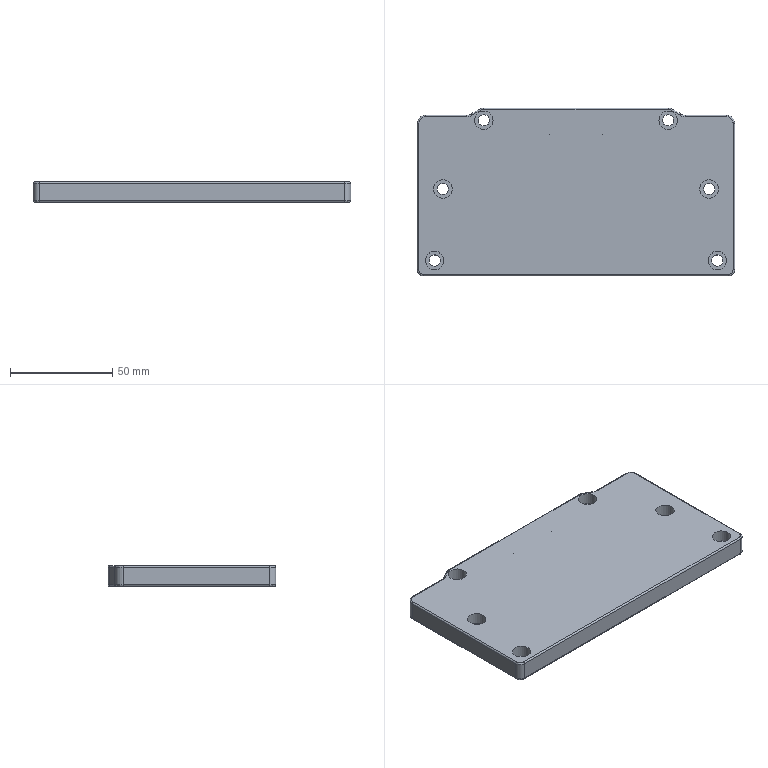Part | STEP file | 1 solid | 72 faces | box 155 x 82 x 10 mm | volume 121887 mm3 | cylinder 38 | plane 16 | spline 16 | cone 2 | commonest cylinder face diameters 1.5 x16 5.5 x6 8 x6 9 x6 3.3 x2 6 x2